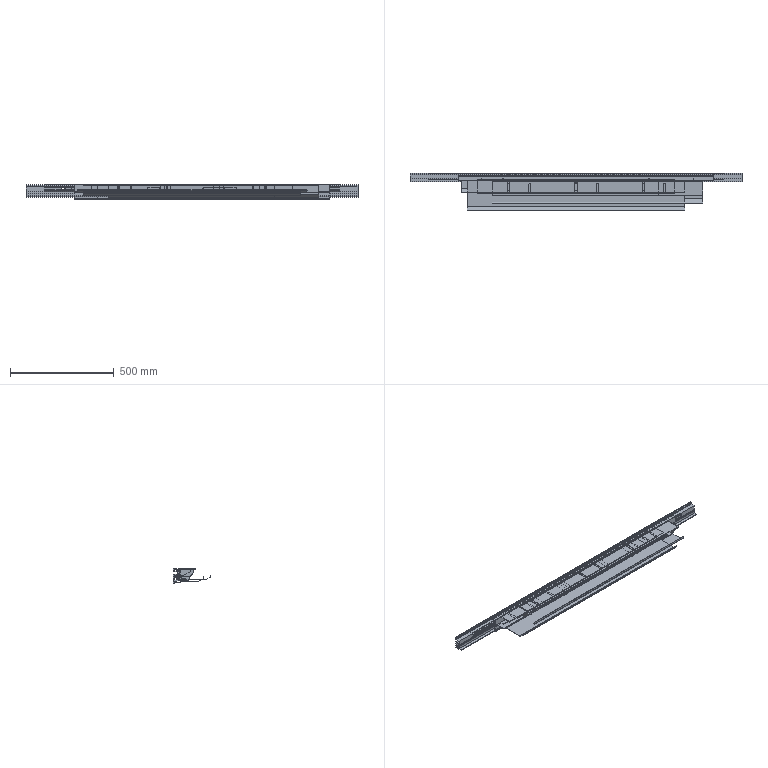Part | 30 solids | 971 faces | box 1600 x 178.321 x 70 mm | volume 5108004 mm3 | plane 651 | cylinder 320 | commonest cylinder face diameters 10 x95 9 x42 6 x39 7 x39 2 x36 3 x18